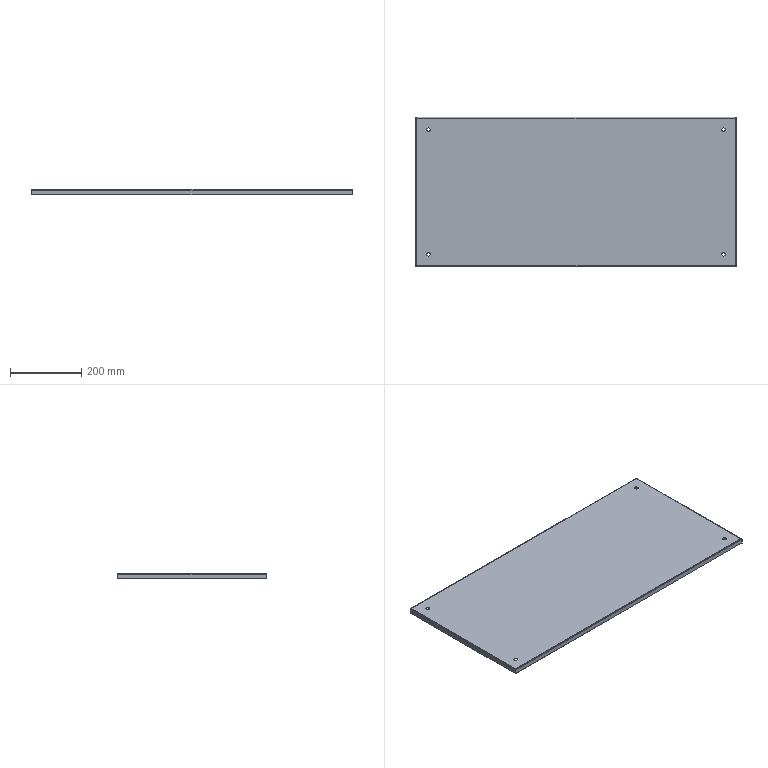Part | 1 solid | 46 faces | box 900 x 420 x 15 mm | volume 617319 mm3 | plane 22 | cylinder 16 | spline 8 | commonest cylinder face diameters 10 x8 1.473 x4 4.473 x4